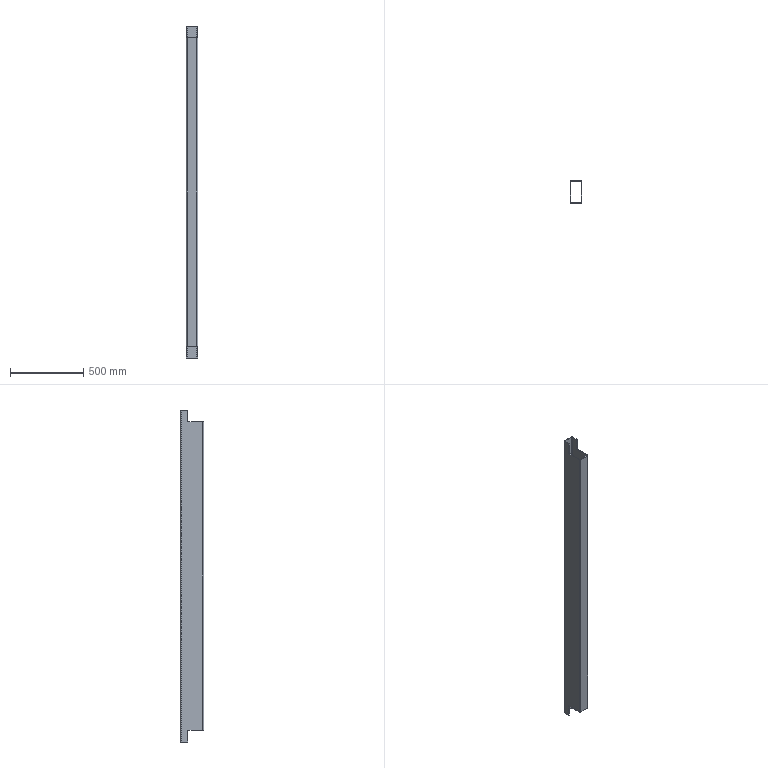Part | STEP file | 750078112 | 1 solid | 24 faces | box 80 x 160 x 2272 mm | volume 4914158 mm3 | plane 16 | cylinder 8 | commonest cylinder face diameters 4 x4 14 x4
STEP:
#1=CARTESIAN_POINT('',(-35.,-73.,1057.));
#2=VERTEX_POINT('',#1);
#3=CARTESIAN_POINT('',(-35.,28.5,1057.));
#4=VERTEX_POINT('',#3);
#5=CARTESIAN_POINT('',(-35.,-73.,1057.));
#6=DIRECTION('',(0.,1.,0.));
#7=VECTOR('',#6,1000.);
#8=LINE('',#5,#7);
#9=EDGE_CURVE('',#2,#4,#8,.T.);
#10=ORIENTED_EDGE('',*,*,#9,.F.);
#11=CARTESIAN_POINT('',(-35.,-73.,-1057.));
#12=VERTEX_POINT('',#11);
#13=CARTESIAN_POINT('',(-35.,-73.,1136.));
#14=DIRECTION('',(0.,0.,1.));
#15=VECTOR('',#14,1000.);
#16=LINE('',#13,#15);
#17=EDGE_CURVE('',#12,#2,#16,.T.);
#18=ORIENTED_EDGE('',*,*,#17,.F.);
#19=CARTESIAN_POINT('',(-35.,28.5,-1057.));
#20=VERTEX_POINT('',#19);
#21=CARTESIAN_POINT('',(-35.,-73.,-1057.));
#22=DIRECTION('',(0.,-1.,0.));
#23=VECTOR('',#22,1000.);
#24=LINE('',#21,#23);
#25=EDGE_CURVE('',#20,#12,#24,.T.);
#26=ORIENTED_EDGE('',*,*,#25,.F.);
#27=CARTESIAN_POINT('',(-35.,28.5,-1136.));
#28=VERTEX_POINT('',#27);
#29=CARTESIAN_POINT('',(-35.,28.5,1136.));
#30=DIRECTION('',(0.,0.,1.));
#31=VECTOR('',#30,1000.);
#32=LINE('',#29,#31);
#33=EDGE_CURVE('',#28,#20,#32,.T.);
#34=ORIENTED_EDGE('',*,*,#33,.F.);
#35=CARTESIAN_POINT('',(-35.,73.,-1136.));
#36=VERTEX_POINT('',#35);
#37=CARTESIAN_POINT('',(-35.,-73.,-1136.));
#38=DIRECTION('',(0.,-1.,0.));
#39=VECTOR('',#38,1000.);
#40=LINE('',#37,#39);
#41=EDGE_CURVE('',#36,#28,#40,.T.);
#42=ORIENTED_EDGE('',*,*,#41,.F.);
#43=CARTESIAN_POINT('',(-35.,73.,1136.));
#44=VERTEX_POINT('',#43);
#45=CARTESIAN_POINT('',(-35.,73.,1136.));
#46=DIRECTION('',(0.,0.,-1.));
#47=VECTOR('',#46,1000.);
#48=LINE('',#45,#47);
#49=EDGE_CURVE('',#44,#36,#48,.T.);
#50=ORIENTED_EDGE('',*,*,#49,.F.);
#51=CARTESIAN_POINT('',(-35.,28.5,1136.));
#52=VERTEX_POINT('',#51);
#53=CARTESIAN_POINT('',(-35.,-73.,1136.));
#54=DIRECTION('',(0.,1.,0.));
#55=VECTOR('',#54,1000.);
#56=LINE('',#53,#55);
#57=EDGE_CURVE('',#52,#44,#56,.T.);
#58=ORIENTED_EDGE('',*,*,#57,.F.);
#59=CARTESIAN_POINT('',(-35.,28.5,1136.));
#60=DIRECTION('',(0.,0.,1.));
#61=VECTOR('',#60,1000.);
#62=LINE('',#59,#61);
#63=EDGE_CURVE('',#4,#52,#62,.T.);
#64=ORIENTED_EDGE('',*,*,#63,.F.);
#65=EDGE_LOOP('',(#10,#18,#26,#34,#42,#50,#58,#64));
#66=FACE_OUTER_BOUND('',#65,.T.);
#67=CARTESIAN_POINT('',(-35.,-73.,1136.));
#68=DIRECTION('',(-1.,0.,0.));
#69=DIRECTION('',(0.,-1.,0.));
#70=AXIS2_PLACEMENT_3D('',#67,#68,#69);
#71=PLANE('',#70);
#72=ADVANCED_FACE('',(#66),#71,.F.);
#73=CARTESIAN_POINT('',(-40.,28.5,1057.));
#74=VERTEX_POINT('',#73);
#75=CARTESIAN_POINT('',(-40.,28.5,1136.));
#76=VERTEX_POINT('',#75);
#77=CARTESIAN_POINT('',(-40.,28.5,1057.));
#78=DIRECTION('',(0.,0.,1.));
#79=VECTOR('',#78,1000.);
#80=LINE('',#77,#79);
#81=EDGE_CURVE('',#74,#76,#80,.T.);
#82=ORIENTED_EDGE('',*,*,#81,.F.);
#83=CARTESIAN_POINT('',(-54960.,28.5,1057.));
#84=DIRECTION('',(-1.,0.,0.));
#85=VECTOR('',#84,1000.);
#86=LINE('',#83,#85);
#87=EDGE_CURVE('',#4,#74,#86,.T.);
#88=ORIENTED_EDGE('',*,*,#87,.F.);
#89=ORIENTED_EDGE('',*,*,#63,.T.);
#90=CARTESIAN_POINT('',(-54960.,28.5,1136.));
#91=DIRECTION('',(1.,0.,0.));
#92=VECTOR('',#91,1000.);
#93=LINE('',#90,#92);
#94=EDGE_CURVE('',#76,#52,#93,.T.);
#95=ORIENTED_EDGE('',*,*,#94,.F.);
#96=EDGE_LOOP('',(#82,#88,#89,#95));
#97=FACE_OUTER_BOUND('',#96,.T.);
#98=CARTESIAN_POINT('',(-54960.,28.5,1057.));
#99=DIRECTION('',(0.,1.,0.));
#100=DIRECTION('',(-1.,0.,0.));
#101=AXIS2_PLACEMENT_3D('',#98,#99,#100);
#102=PLANE('',#101);
#103=ADVANCED_FACE('',(#97),#102,.F.);
#104=CARTESIAN_POINT('',(-40.,-73.,1057.));
#105=VERTEX_POINT('',#104);
#106=CARTESIAN_POINT('',(-40.,-80.,1057.));
#107=DIRECTION('',(0.,1.,0.));
#108=VECTOR('',#107,1000.);
#109=LINE('',#106,#108);
#110=EDGE_CURVE('',#105,#74,#109,.T.);
#111=ORIENTED_EDGE('',*,*,#110,.F.);
#112=CARTESIAN_POINT('',(-33.,-80.,1057.));
#113=VERTEX_POINT('',#112);
#114=CARTESIAN_POINT('',(-33.,-73.,1057.));
#115=DIRECTION('',(0.,0.,-1.));
#116=DIRECTION('',(-1.,0.,0.));
#117=AXIS2_PLACEMENT_3D('',#114,#115,#116);
#118=CIRCLE('',#117,7.);
#119=EDGE_CURVE('',#113,#105,#118,.T.);
#120=ORIENTED_EDGE('',*,*,#119,.F.);
#121=CARTESIAN_POINT('',(33.,-80.,1057.));
#122=VERTEX_POINT('',#121);
#123=CARTESIAN_POINT('',(-54960.,-80.,1057.));
#124=DIRECTION('',(-1.,0.,0.));
#125=VECTOR('',#124,1000.);
#126=LINE('',#123,#125);
#127=EDGE_CURVE('',#122,#113,#126,.T.);
#128=ORIENTED_EDGE('',*,*,#127,.F.);
#129=CARTESIAN_POINT('',(40.,-73.,1057.));
#130=VERTEX_POINT('',#129);
#131=CARTESIAN_POINT('',(33.,-73.,1057.));
#132=DIRECTION('',(0.,0.,-1.));
#133=DIRECTION('',(-1.,0.,0.));
#134=AXIS2_PLACEMENT_3D('',#131,#132,#133);
#135=CIRCLE('',#134,7.);
#136=EDGE_CURVE('',#130,#122,#135,.T.);
#137=ORIENTED_EDGE('',*,*,#136,.F.);
#138=CARTESIAN_POINT('',(40.,28.5,1057.));
#139=VERTEX_POINT('',#138);
#140=CARTESIAN_POINT('',(40.,-80.,1057.));
#141=DIRECTION('',(0.,-1.,0.));
#142=VECTOR('',#141,1000.);
#143=LINE('',#140,#142);
#144=EDGE_CURVE('',#139,#130,#143,.T.);
#145=ORIENTED_EDGE('',*,*,#144,.F.);
#146=CARTESIAN_POINT('',(35.,28.5,1057.));
#147=VERTEX_POINT('',#146);
#148=CARTESIAN_POINT('',(-54960.,28.5,1057.));
#149=DIRECTION('',(1.,0.,0.));
#150=VECTOR('',#149,1000.);
#151=LINE('',#148,#150);
#152=EDGE_CURVE('',#147,#139,#151,.T.);
#153=ORIENTED_EDGE('',*,*,#152,.F.);
#154=CARTESIAN_POINT('',(35.,-73.,1057.));
#155=VERTEX_POINT('',#154);
#156=CARTESIAN_POINT('',(35.,-80.,1057.));
#157=DIRECTION('',(0.,1.,0.));
#158=VECTOR('',#157,1000.);
#159=LINE('',#156,#158);
#160=EDGE_CURVE('',#155,#147,#159,.T.);
#161=ORIENTED_EDGE('',*,*,#160,.F.);
#162=CARTESIAN_POINT('',(33.,-75.,1057.));
#163=VERTEX_POINT('',#162);
#164=CARTESIAN_POINT('',(33.,-73.,1057.));
#165=DIRECTION('',(0.,0.,1.));
#166=DIRECTION('',(-1.,0.,0.));
#167=AXIS2_PLACEMENT_3D('',#164,#165,#166);
#168=CIRCLE('',#167,2.);
#169=EDGE_CURVE('',#163,#155,#168,.T.);
#170=ORIENTED_EDGE('',*,*,#169,.F.);
#171=CARTESIAN_POINT('',(-33.,-75.,1057.));
#172=VERTEX_POINT('',#171);
#173=CARTESIAN_POINT('',(-54960.,-75.,1057.));
#174=DIRECTION('',(1.,0.,0.));
#175=VECTOR('',#174,1000.);
#176=LINE('',#173,#175);
#177=EDGE_CURVE('',#172,#163,#176,.T.);
#178=ORIENTED_EDGE('',*,*,#177,.F.);
#179=CARTESIAN_POINT('',(-33.,-73.,1057.));
#180=DIRECTION('',(0.,0.,1.));
#181=DIRECTION('',(-1.,0.,0.));
#182=AXIS2_PLACEMENT_3D('',#179,#180,#181);
#183=CIRCLE('',#182,2.);
#184=EDGE_CURVE('',#2,#172,#183,.T.);
#185=ORIENTED_EDGE('',*,*,#184,.F.);
#186=ORIENTED_EDGE('',*,*,#9,.T.);
#187=ORIENTED_EDGE('',*,*,#87,.T.);
#188=EDGE_LOOP('',(#111,#120,#128,#137,#145,#153,#161,#170,#178,#185,#186,#187));
#189=FACE_OUTER_BOUND('',#188,.T.);
#190=CARTESIAN_POINT('',(-54960.,-80.,1057.));
#191=DIRECTION('',(0.,0.,-1.));
#192=DIRECTION('',(0.,1.,0.));
#193=AXIS2_PLACEMENT_3D('',#190,#191,#192);
#194=PLANE('',#193);
#195=ADVANCED_FACE('',(#189),#194,.F.);
#196=ORIENTED_EDGE('',*,*,#184,.T.);
#197=CARTESIAN_POINT('',(-33.,-75.,-1057.));
#198=VERTEX_POINT('',#197);
#199=CARTESIAN_POINT('',(-33.,-75.,1136.));
#200=DIRECTION('',(0.,0.,1.));
#201=VECTOR('',#200,1000.);
#202=LINE('',#199,#201);
#203=EDGE_CURVE('',#198,#172,#202,.T.);
#204=ORIENTED_EDGE('',*,*,#203,.F.);
#205=CARTESIAN_POINT('',(-33.,-73.,-1057.));
#206=DIRECTION('',(0.,0.,1.));
#207=DIRECTION('',(-1.,0.,0.));
#208=AXIS2_PLACEMENT_3D('',#205,#206,#207);
#209=CIRCLE('',#208,2.);
#210=EDGE_CURVE('',#12,#198,#209,.T.);
#211=ORIENTED_EDGE('',*,*,#210,.F.);
#212=ORIENTED_EDGE('',*,*,#17,.T.);
#213=EDGE_LOOP('',(#196,#204,#211,#212));
#214=FACE_OUTER_BOUND('',#213,.T.);
#215=CARTESIAN_POINT('',(-33.,-73.,1136.));
#216=DIRECTION('',(0.,0.,-1.));
#217=DIRECTION('',(-1.,0.,0.));
#218=AXIS2_PLACEMENT_3D('',#215,#216,#217);
#219=CYLINDRICAL_SURFACE('',#218,2.);
#220=ADVANCED_FACE('',(#214),#219,.F.);
#221=CARTESIAN_POINT('',(33.,-75.,-1057.));
#222=VERTEX_POINT('',#221);
#223=CARTESIAN_POINT('',(-54960.,-75.,-1057.));
#224=DIRECTION('',(-1.,0.,0.));
#225=VECTOR('',#224,1000.);
#226=LINE('',#223,#225);
#227=EDGE_CURVE('',#222,#198,#226,.T.);
#228=ORIENTED_EDGE('',*,*,#227,.F.);
#229=CARTESIAN_POINT('',(35.,-73.,-1057.));
#230=VERTEX_POINT('',#229);
#231=CARTESIAN_POINT('',(33.,-73.,-1057.));
#232=DIRECTION('',(0.,0.,-1.));
#233=DIRECTION('',(-1.,0.,0.));
#234=AXIS2_PLACEMENT_3D('',#231,#232,#233);
#235=CIRCLE('',#234,2.);
#236=EDGE_CURVE('',#230,#222,#235,.T.);
#237=ORIENTED_EDGE('',*,*,#236,.F.);
#238=CARTESIAN_POINT('',(35.,28.5,-1057.));
#239=VERTEX_POINT('',#238);
#240=CARTESIAN_POINT('',(35.,28.5,-1057.));
#241=DIRECTION('',(0.,-1.,0.));
#242=VECTOR('',#241,1000.);
#243=LINE('',#240,#242);
#244=EDGE_CURVE('',#239,#230,#243,.T.);
#245=ORIENTED_EDGE('',*,*,#244,.F.);
#246=CARTESIAN_POINT('',(40.,28.5,-1057.));
#247=VERTEX_POINT('',#246);
#248=CARTESIAN_POINT('',(-54960.,28.5,-1057.));
#249=DIRECTION('',(-1.,0.,0.));
#250=VECTOR('',#249,1000.);
#251=LINE('',#248,#250);
#252=EDGE_CURVE('',#247,#239,#251,.T.);
#253=ORIENTED_EDGE('',*,*,#252,.F.);
#254=CARTESIAN_POINT('',(40.,-73.,-1057.));
#255=VERTEX_POINT('',#254);
#256=CARTESIAN_POINT('',(40.,28.5,-1057.));
#257=DIRECTION('',(0.,1.,0.));
#258=VECTOR('',#257,1000.);
#259=LINE('',#256,#258);
#260=EDGE_CURVE('',#255,#247,#259,.T.);
#261=ORIENTED_EDGE('',*,*,#260,.F.);
#262=CARTESIAN_POINT('',(33.,-80.,-1057.));
#263=VERTEX_POINT('',#262);
#264=CARTESIAN_POINT('',(33.,-73.,-1057.));
#265=DIRECTION('',(0.,0.,1.));
#266=DIRECTION('',(-1.,0.,0.));
#267=AXIS2_PLACEMENT_3D('',#264,#265,#266);
#268=CIRCLE('',#267,7.);
#269=EDGE_CURVE('',#263,#255,#268,.T.);
#270=ORIENTED_EDGE('',*,*,#269,.F.);
#271=CARTESIAN_POINT('',(-33.,-80.,-1057.));
#272=VERTEX_POINT('',#271);
#273=CARTESIAN_POINT('',(-54960.,-80.,-1057.));
#274=DIRECTION('',(1.,0.,0.));
#275=VECTOR('',#274,1000.);
#276=LINE('',#273,#275);
#277=EDGE_CURVE('',#272,#263,#276,.T.);
#278=ORIENTED_EDGE('',*,*,#277,.F.);
#279=CARTESIAN_POINT('',(-40.,-73.,-1057.));
#280=VERTEX_POINT('',#279);
#281=CARTESIAN_POINT('',(-33.,-73.,-1057.));
#282=DIRECTION('',(0.,0.,1.));
#283=DIRECTION('',(-1.,0.,0.));
#284=AXIS2_PLACEMENT_3D('',#281,#282,#283);
#285=CIRCLE('',#284,7.);
#286=EDGE_CURVE('',#280,#272,#285,.T.);
#287=ORIENTED_EDGE('',*,*,#286,.F.);
#288=CARTESIAN_POINT('',(-40.,28.5,-1057.));
#289=VERTEX_POINT('',#288);
#290=CARTESIAN_POINT('',(-40.,28.5,-1057.));
#291=DIRECTION('',(0.,-1.,0.));
#292=VECTOR('',#291,1000.);
#293=LINE('',#290,#292);
#294=EDGE_CURVE('',#289,#280,#293,.T.);
#295=ORIENTED_EDGE('',*,*,#294,.F.);
#296=CARTESIAN_POINT('',(-54960.,28.5,-1057.));
#297=DIRECTION('',(-1.,0.,0.));
#298=VECTOR('',#297,1000.);
#299=LINE('',#296,#298);
#300=EDGE_CURVE('',#20,#289,#299,.T.);
#301=ORIENTED_EDGE('',*,*,#300,.F.);
#302=ORIENTED_EDGE('',*,*,#25,.T.);
#303=ORIENTED_EDGE('',*,*,#210,.T.);
#304=EDGE_LOOP('',(#228,#237,#245,#253,#261,#270,#278,#287,#295,#301,#302,#303));
#305=FACE_OUTER_BOUND('',#304,.T.);
#306=CARTESIAN_POINT('',(-54960.,28.5,-1057.));
#307=DIRECTION('',(0.,0.,1.));
#308=DIRECTION('',(0.,-1.,0.));
#309=AXIS2_PLACEMENT_3D('',#306,#307,#308);
#310=PLANE('',#309);
#311=ADVANCED_FACE('',(#305),#310,.F.);
#312=CARTESIAN_POINT('',(-40.,28.5,-1136.));
#313=VERTEX_POINT('',#312);
#314=CARTESIAN_POINT('',(-40.,28.5,-1136.));
#315=DIRECTION('',(0.,0.,1.));
#316=VECTOR('',#315,1000.);
#317=LINE('',#314,#316);
#318=EDGE_CURVE('',#313,#289,#317,.T.);
#319=ORIENTED_EDGE('',*,*,#318,.F.);
#320=CARTESIAN_POINT('',(-54960.,28.5,-1136.));
#321=DIRECTION('',(-1.,0.,0.));
#322=VECTOR('',#321,1000.);
#323=LINE('',#320,#322);
#324=EDGE_CURVE('',#28,#313,#323,.T.);
#325=ORIENTED_EDGE('',*,*,#324,.F.);
#326=ORIENTED_EDGE('',*,*,#33,.T.);
#327=ORIENTED_EDGE('',*,*,#300,.T.);
#328=EDGE_LOOP('',(#319,#325,#326,#327));
#329=FACE_OUTER_BOUND('',#328,.T.);
#330=CARTESIAN_POINT('',(-54960.,28.5,-1136.));
#331=DIRECTION('',(0.,1.,0.));
#332=DIRECTION('',(-1.,0.,0.));
#333=AXIS2_PLACEMENT_3D('',#330,#331,#332);
#334=PLANE('',#333);
#335=ADVANCED_FACE('',(#329),#334,.F.);
#336=CARTESIAN_POINT('',(-33.,75.,-1136.));
#337=VERTEX_POINT('',#336);
#338=CARTESIAN_POINT('',(-33.,73.,-1136.));
#339=DIRECTION('',(0.,0.,1.));
#340=DIRECTION('',(-1.,0.,0.));
#341=AXIS2_PLACEMENT_3D('',#338,#339,#340);
#342=CIRCLE('',#341,2.);
#343=EDGE_CURVE('',#337,#36,#342,.T.);
#344=ORIENTED_EDGE('',*,*,#343,.T.);
#345=ORIENTED_EDGE('',*,*,#41,.T.);
#346=ORIENTED_EDGE('',*,*,#324,.T.);
#347=CARTESIAN_POINT('',(-40.,73.,-1136.));
#348=VERTEX_POINT('',#347);
#349=CARTESIAN_POINT('',(-40.,-73.,-1136.));
#350=DIRECTION('',(0.,1.,0.));
#351=VECTOR('',#350,1000.);
#352=LINE('',#349,#351);
#353=EDGE_CURVE('',#313,#348,#352,.T.);
#354=ORIENTED_EDGE('',*,*,#353,.T.);
#355=CARTESIAN_POINT('',(-33.,80.,-1136.));
#356=VERTEX_POINT('',#355);
#357=CARTESIAN_POINT('',(-33.,73.,-1136.));
#358=DIRECTION('',(0.,0.,-1.));
#359=DIRECTION('',(-1.,0.,0.));
#360=AXIS2_PLACEMENT_3D('',#357,#358,#359);
#361=CIRCLE('',#360,7.);
#362=EDGE_CURVE('',#348,#356,#361,.T.);
#363=ORIENTED_EDGE('',*,*,#362,.T.);
#364=CARTESIAN_POINT('',(33.,80.,-1136.));
#365=VERTEX_POINT('',#364);
#366=CARTESIAN_POINT('',(33.,80.,-1136.));
#367=DIRECTION('',(1.,0.,0.));
#368=VECTOR('',#367,1000.);
#369=LINE('',#366,#368);
#370=EDGE_CURVE('',#356,#365,#369,.T.);
#371=ORIENTED_EDGE('',*,*,#370,.T.);
#372=CARTESIAN_POINT('',(40.,73.,-1136.));
#373=VERTEX_POINT('',#372);
#374=CARTESIAN_POINT('',(33.,73.,-1136.));
#375=DIRECTION('',(0.,0.,-1.));
#376=DIRECTION('',(-1.,0.,0.));
#377=AXIS2_PLACEMENT_3D('',#374,#375,#376);
#378=CIRCLE('',#377,7.);
#379=EDGE_CURVE('',#365,#373,#378,.T.);
#380=ORIENTED_EDGE('',*,*,#379,.T.);
#381=CARTESIAN_POINT('',(40.,28.5,-1136.));
#382=VERTEX_POINT('',#381);
#383=CARTESIAN_POINT('',(40.,-73.,-1136.));
#384=DIRECTION('',(0.,-1.,0.));
#385=VECTOR('',#384,1000.);
#386=LINE('',#383,#385);
#387=EDGE_CURVE('',#373,#382,#386,.T.);
#388=ORIENTED_EDGE('',*,*,#387,.T.);
#389=CARTESIAN_POINT('',(35.,28.5,-1136.));
#390=VERTEX_POINT('',#389);
#391=CARTESIAN_POINT('',(33.,28.5,-1136.));
#392=DIRECTION('',(-1.,0.,0.));
#393=VECTOR('',#392,1000.);
#394=LINE('',#391,#393);
#395=EDGE_CURVE('',#382,#390,#394,.T.);
#396=ORIENTED_EDGE('',*,*,#395,.T.);
#397=CARTESIAN_POINT('',(35.,73.,-1136.));
#398=VERTEX_POINT('',#397);
#399=CARTESIAN_POINT('',(35.,-73.,-1136.));
#400=DIRECTION('',(0.,1.,0.));
#401=VECTOR('',#400,1000.);
#402=LINE('',#399,#401);
#403=EDGE_CURVE('',#390,#398,#402,.T.);
#404=ORIENTED_EDGE('',*,*,#403,.T.);
#405=CARTESIAN_POINT('',(33.,75.,-1136.));
#406=VERTEX_POINT('',#405);
#407=CARTESIAN_POINT('',(33.,73.,-1136.));
#408=DIRECTION('',(0.,0.,1.));
#409=DIRECTION('',(-1.,0.,0.));
#410=AXIS2_PLACEMENT_3D('',#407,#408,#409);
#411=CIRCLE('',#410,2.);
#412=EDGE_CURVE('',#398,#406,#411,.T.);
#413=ORIENTED_EDGE('',*,*,#412,.T.);
#414=CARTESIAN_POINT('',(33.,75.,-1136.));
#415=DIRECTION('',(-1.,0.,0.));
#416=VECTOR('',#415,1000.);
#417=LINE('',#414,#416);
#418=EDGE_CURVE('',#406,#337,#417,.T.);
#419=ORIENTED_EDGE('',*,*,#418,.T.);
#420=EDGE_LOOP('',(#344,#345,#346,#354,#363,#371,#380,#388,#396,#404,#413,#419));
#421=FACE_OUTER_BOUND('',#420,.T.);
#422=CARTESIAN_POINT('',(33.,-73.,-1136.));
#423=DIRECTION('',(0.,0.,-1.));
#424=DIRECTION('',(-1.,0.,0.));
#425=AXIS2_PLACEMENT_3D('',#422,#423,#424);
#426=PLANE('',#425);
#427=ADVANCED_FACE('',(#421),#426,.T.);
#428=CARTESIAN_POINT('',(-33.,75.,1136.));
#429=VERTEX_POINT('',#428);
#430=CARTESIAN_POINT('',(-33.,75.,1136.));
#431=DIRECTION('',(0.,0.,-1.));
#432=VECTOR('',#431,1000.);
#433=LINE('',#430,#432);
#434=EDGE_CURVE('',#429,#337,#433,.T.);
#435=ORIENTED_EDGE('',*,*,#434,.F.);
#436=CARTESIAN_POINT('',(-33.,73.,1136.));
#437=DIRECTION('',(0.,0.,-1.));
#438=DIRECTION('',(-1.,0.,0.));
#439=AXIS2_PLACEMENT_3D('',#436,#437,#438);
#440=CIRCLE('',#439,2.);
#441=EDGE_CURVE('',#44,#429,#440,.T.);
#442=ORIENTED_EDGE('',*,*,#441,.F.);
#443=ORIENTED_EDGE('',*,*,#49,.T.);
#444=ORIENTED_EDGE('',*,*,#343,.F.);
#445=EDGE_LOOP('',(#435,#442,#443,#444));
#446=FACE_OUTER_BOUND('',#445,.T.);
#447=CARTESIAN_POINT('',(-33.,73.,1136.));
#448=DIRECTION('',(0.,0.,-1.));
#449=DIRECTION('',(-1.,0.,0.));
#450=AXIS2_PLACEMENT_3D('',#447,#448,#449);
#451=CYLINDRICAL_SURFACE('',#450,2.);
#452=ADVANCED_FACE('',(#446),#451,.F.);
#453=ORIENTED_EDGE('',*,*,#94,.T.);
#454=ORIENTED_EDGE('',*,*,#57,.T.);
#455=ORIENTED_EDGE('',*,*,#441,.T.);
#456=CARTESIAN_POINT('',(33.,75.,1136.));
#457=VERTEX_POINT('',#456);
#458=CARTESIAN_POINT('',(33.,75.,1136.));
#459=DIRECTION('',(-1.,0.,0.));
#460=VECTOR('',#459,1000.);
#461=LINE('',#458,#460);
#462=EDGE_CURVE('',#457,#429,#461,.T.);
#463=ORIENTED_EDGE('',*,*,#462,.F.);
#464=CARTESIAN_POINT('',(35.,73.,1136.));
#465=VERTEX_POINT('',#464);
#466=CARTESIAN_POINT('',(33.,73.,1136.));
#467=DIRECTION('',(0.,0.,1.));
#468=DIRECTION('',(-1.,0.,0.));
#469=AXIS2_PLACEMENT_3D('',#466,#467,#468);
#470=CIRCLE('',#469,2.);
#471=EDGE_CURVE('',#465,#457,#470,.T.);
#472=ORIENTED_EDGE('',*,*,#471,.F.);
#473=CARTESIAN_POINT('',(35.,28.5,1136.));
#474=VERTEX_POINT('',#473);
#475=CARTESIAN_POINT('',(35.,-73.,1136.));
#476=DIRECTION('',(0.,1.,0.));
#477=VECTOR('',#476,1000.);
#478=LINE('',#475,#477);
#479=EDGE_CURVE('',#474,#465,#478,.T.);
#480=ORIENTED_EDGE('',*,*,#479,.F.);
#481=CARTESIAN_POINT('',(40.,28.5,1136.));
#482=VERTEX_POINT('',#481);
#483=CARTESIAN_POINT('',(33.,28.5,1136.));
#484=DIRECTION('',(-1.,0.,0.));
#485=VECTOR('',#484,1000.);
#486=LINE('',#483,#485);
#487=EDGE_CURVE('',#482,#474,#486,.T.);
#488=ORIENTED_EDGE('',*,*,#487,.F.);
#489=CARTESIAN_POINT('',(40.,73.,1136.));
#490=VERTEX_POINT('',#489);
#491=CARTESIAN_POINT('',(40.,-73.,1136.));
#492=DIRECTION('',(0.,-1.,0.));
#493=VECTOR('',#492,1000.);
#494=LINE('',#491,#493);
#495=EDGE_CURVE('',#490,#482,#494,.T.);
#496=ORIENTED_EDGE('',*,*,#495,.F.);
#497=CARTESIAN_POINT('',(33.,80.,1136.));
#498=VERTEX_POINT('',#497);
#499=CARTESIAN_POINT('',(33.,73.,1136.));
#500=DIRECTION('',(0.,0.,-1.));
#501=DIRECTION('',(-1.,0.,0.));
#502=AXIS2_PLACEMENT_3D('',#499,#500,#501);
#503=CIRCLE('',#502,7.);
#504=EDGE_CURVE('',#498,#490,#503,.T.);
#505=ORIENTED_EDGE('',*,*,#504,.F.);
#506=CARTESIAN_POINT('',(-33.,80.,1136.));
#507=VERTEX_POINT('',#506);
#508=CARTESIAN_POINT('',(33.,80.,1136.));
#509=DIRECTION('',(1.,0.,0.));
#510=VECTOR('',#509,1000.);
#511=LINE('',#508,#510);
#512=EDGE_CURVE('',#507,#498,#511,.T.);
#513=ORIENTED_EDGE('',*,*,#512,.F.);
#514=CARTESIAN_POINT('',(-40.,73.,1136.));
#515=VERTEX_POINT('',#514);
#516=CARTESIAN_POINT('',(-33.,73.,1136.));
#517=DIRECTION('',(0.,0.,-1.));
#518=DIRECTION('',(-1.,0.,0.));
#519=AXIS2_PLACEMENT_3D('',#516,#517,#518);
#520=CIRCLE('',#519,7.);
#521=EDGE_CURVE('',#515,#507,#520,.T.);
#522=ORIENTED_EDGE('',*,*,#521,.F.);
#523=CARTESIAN_POINT('',(-40.,-73.,1136.));
#524=DIRECTION('',(0.,1.,0.));
#525=VECTOR('',#524,1000.);
#526=LINE('',#523,#525);
#527=EDGE_CURVE('',#76,#515,#526,.T.);
#528=ORIENTED_EDGE('',*,*,#527,.F.);
#529=EDGE_LOOP('',(#453,#454,#455,#463,#472,#480,#488,#496,#505,#513,#522,#528));
#530=FACE_OUTER_BOUND('',#529,.T.);
#531=CARTESIAN_POINT('',(33.,-73.,1136.));
#532=DIRECTION('',(0.,0.,-1.));
#533=DIRECTION('',(-1.,0.,0.));
#534=AXIS2_PLACEMENT_3D('',#531,#532,#533);
#535=PLANE('',#534);
#536=ADVANCED_FACE('',(#530),#535,.F.);
#537=ORIENTED_EDGE('',*,*,#294,.T.);
#538=CARTESIAN_POINT('',(-40.,-73.,1136.));
#539=DIRECTION('',(0.,0.,1.));
#540=VECTOR('',#539,1000.);
#541=LINE('',#538,#540);
#542=EDGE_CURVE('',#280,#105,#541,.T.);
#543=ORIENTED_EDGE('',*,*,#542,.T.);
#544=ORIENTED_EDGE('',*,*,#110,.T.);
#545=ORIENTED_EDGE('',*,*,#81,.T.);
#546=ORIENTED_EDGE('',*,*,#527,.T.);
#547=CARTESIAN_POINT('',(-40.,73.,1136.));
#548=DIRECTION('',(0.,0.,-1.));
#549=VECTOR('',#548,1000.);
#550=LINE('',#547,#549);
#551=EDGE_CURVE('',#515,#348,#550,.T.);
#552=ORIENTED_EDGE('',*,*,#551,.T.);
#553=ORIENTED_EDGE('',*,*,#353,.F.);
#554=ORIENTED_EDGE('',*,*,#318,.T.);
#555=EDGE_LOOP('',(#537,#543,#544,#545,#546,#552,#553,#554));
#556=FACE_OUTER_BOUND('',#555,.T.);
#557=CARTESIAN_POINT('',(-40.,-73.,1136.));
#558=DIRECTION('',(-1.,0.,0.));
#559=DIRECTION('',(0.,0.,1.));
#560=AXIS2_PLACEMENT_3D('',#557,#558,#559);
#561=PLANE('',#560);
#562=ADVANCED_FACE('',(#556),#561,.T.);
#563=ORIENTED_EDGE('',*,*,#286,.T.);
#564=CARTESIAN_POINT('',(-33.,-80.,1136.));
#565=DIRECTION('',(0.,0.,1.));
#566=VECTOR('',#565,1000.);
#567=LINE('',#564,#566);
#568=EDGE_CURVE('',#272,#113,#567,.T.);
#569=ORIENTED_EDGE('',*,*,#568,.T.);
#570=ORIENTED_EDGE('',*,*,#119,.T.);
#571=ORIENTED_EDGE('',*,*,#542,.F.);
#572=EDGE_LOOP('',(#563,#569,#570,#571));
#573=FACE_OUTER_BOUND('',#572,.T.);
#574=CARTESIAN_POINT('',(-33.,-73.,1136.));
#575=DIRECTION('',(0.,0.,-1.));
#576=DIRECTION('',(-1.,0.,0.));
#577=AXIS2_PLACEMENT_3D('',#574,#575,#576);
#578=CYLINDRICAL_SURFACE('',#577,7.);
#579=ADVANCED_FACE('',(#573),#578,.T.);
#580=ORIENTED_EDGE('',*,*,#277,.T.);
#581=CARTESIAN_POINT('',(33.,-80.,1136.));
#582=DIRECTION('',(0.,0.,1.));
#583=VECTOR('',#582,1000.);
#584=LINE('',#581,#583);
#585=EDGE_CURVE('',#263,#122,#584,.T.);
#586=ORIENTED_EDGE('',*,*,#585,.T.);
#587=ORIENTED_EDGE('',*,*,#127,.T.);
#588=ORIENTED_EDGE('',*,*,#568,.F.);
#589=EDGE_LOOP('',(#580,#586,#587,#588));
#590=FACE_OUTER_BOUND('',#589,.T.);
#591=CARTESIAN_POINT('',(33.,-80.,1136.));
#592=DIRECTION('',(0.,-1.,0.));
#593=DIRECTION('',(0.,0.,-1.));
#594=AXIS2_PLACEMENT_3D('',#591,#592,#593);
#595=PLANE('',#594);
#596=ADVANCED_FACE('',(#590),#595,.T.);
#597=ORIENTED_EDGE('',*,*,#269,.T.);
#598=CARTESIAN_POINT('',(40.,-73.,1136.));
#599=DIRECTION('',(0.,0.,1.));
#600=VECTOR('',#599,1000.);
#601=LINE('',#598,#600);
#602=EDGE_CURVE('',#255,#130,#601,.T.);
#603=ORIENTED_EDGE('',*,*,#602,.T.);
#604=ORIENTED_EDGE('',*,*,#136,.T.);
#605=ORIENTED_EDGE('',*,*,#585,.F.);
#606=EDGE_LOOP('',(#597,#603,#604,#605));
#607=FACE_OUTER_BOUND('',#606,.T.);
#608=CARTESIAN_POINT('',(33.,-73.,1136.));
#609=DIRECTION('',(0.,0.,-1.));
#610=DIRECTION('',(-1.,0.,0.));
#611=AXIS2_PLACEMENT_3D('',#608,#609,#610);
#612=CYLINDRICAL_SURFACE('',#611,7.);
#613=ADVANCED_FACE('',(#607),#612,.T.);
#614=ORIENTED_EDGE('',*,*,#495,.T.);
#615=CARTESIAN_POINT('',(40.,28.5,1136.));
#616=DIRECTION('',(0.,0.,-1.));
#617=VECTOR('',#616,1000.);
#618=LINE('',#615,#617);
#619=EDGE_CURVE('',#482,#139,#618,.T.);
#620=ORIENTED_EDGE('',*,*,#619,.T.);
#621=ORIENTED_EDGE('',*,*,#144,.T.);
#622=ORIENTED_EDGE('',*,*,#602,.F.);
#623=ORIENTED_EDGE('',*,*,#260,.T.);
#624=CARTESIAN_POINT('',(40.,28.5,1136.));
#625=DIRECTION('',(0.,0.,-1.));
#626=VECTOR('',#625,1000.);
#627=LINE('',#624,#626);
#628=EDGE_CURVE('',#247,#382,#627,.T.);
#629=ORIENTED_EDGE('',*,*,#628,.T.);
#630=ORIENTED_EDGE('',*,*,#387,.F.);
#631=CARTESIAN_POINT('',(40.,73.,1136.));
#632=DIRECTION('',(0.,0.,1.));
#633=VECTOR('',#632,1000.);
#634=LINE('',#631,#633);
#635=EDGE_CURVE('',#373,#490,#634,.T.);
#636=ORIENTED_EDGE('',*,*,#635,.T.);
#637=EDGE_LOOP('',(#614,#620,#621,#622,#623,#629,#630,#636));
#638=FACE_OUTER_BOUND('',#637,.T.);
#639=CARTESIAN_POINT('',(40.,73.,1136.));
#640=DIRECTION('',(1.,0.,0.));
#641=DIRECTION('',(0.,1.,0.));
#642=AXIS2_PLACEMENT_3D('',#639,#640,#641);
#643=PLANE('',#642);
#644=ADVANCED_FACE('',(#638),#643,.T.);
#645=ORIENTED_EDGE('',*,*,#619,.F.);
#646=ORIENTED_EDGE('',*,*,#487,.T.);
#647=CARTESIAN_POINT('',(35.,28.5,1057.));
#648=DIRECTION('',(0.,0.,1.));
#649=VECTOR('',#648,1000.);
#650=LINE('',#647,#649);
#651=EDGE_CURVE('',#147,#474,#650,.T.);
#652=ORIENTED_EDGE('',*,*,#651,.F.);
#653=ORIENTED_EDGE('',*,*,#152,.T.);
#654=EDGE_LOOP('',(#645,#646,#652,#653));
#655=FACE_OUTER_BOUND('',#654,.T.);
#656=CARTESIAN_POINT('',(-54960.,28.5,1057.));
#657=DIRECTION('',(0.,1.,0.));
#658=DIRECTION('',(-1.,0.,0.));
#659=AXIS2_PLACEMENT_3D('',#656,#657,#658);
#660=PLANE('',#659);
#661=ADVANCED_FACE('',(#655),#660,.F.);
#662=ORIENTED_EDGE('',*,*,#160,.T.);
#663=ORIENTED_EDGE('',*,*,#651,.T.);
#664=ORIENTED_EDGE('',*,*,#479,.T.);
#665=CARTESIAN_POINT('',(35.,73.,1136.));
#666=DIRECTION('',(0.,0.,1.));
#667=VECTOR('',#666,1000.);
#668=LINE('',#665,#667);
#669=EDGE_CURVE('',#398,#465,#668,.T.);
#670=ORIENTED_EDGE('',*,*,#669,.F.);
#671=ORIENTED_EDGE('',*,*,#403,.F.);
#672=CARTESIAN_POINT('',(35.,28.5,1136.));
#673=DIRECTION('',(0.,0.,-1.));
#674=VECTOR('',#673,1000.);
#675=LINE('',#672,#674);
#676=EDGE_CURVE('',#239,#390,#675,.T.);
#677=ORIENTED_EDGE('',*,*,#676,.F.);
#678=ORIENTED_EDGE('',*,*,#244,.T.);
#679=CARTESIAN_POINT('',(35.,-73.,1136.));
#680=DIRECTION('',(0.,0.,-1.));
#681=VECTOR('',#680,1000.);
#682=LINE('',#679,#681);
#683=EDGE_CURVE('',#155,#230,#682,.T.);
#684=ORIENTED_EDGE('',*,*,#683,.F.);
#685=EDGE_LOOP('',(#662,#663,#664,#670,#671,#677,#678,#684));
#686=FACE_OUTER_BOUND('',#685,.T.);
#687=CARTESIAN_POINT('',(35.,73.,1136.));
#688=DIRECTION('',(1.,0.,0.));
#689=DIRECTION('',(0.,1.,0.));
#690=AXIS2_PLACEMENT_3D('',#687,#688,#689);
#691=PLANE('',#690);
#692=ADVANCED_FACE('',(#686),#691,.F.);
#693=ORIENTED_EDGE('',*,*,#169,.T.);
#694=ORIENTED_EDGE('',*,*,#683,.T.);
#695=ORIENTED_EDGE('',*,*,#236,.T.);
#696=CARTESIAN_POINT('',(33.,-75.,1136.));
#697=DIRECTION('',(0.,0.,-1.));
#698=VECTOR('',#697,1000.);
#699=LINE('',#696,#698);
#700=EDGE_CURVE('',#163,#222,#699,.T.);
#701=ORIENTED_EDGE('',*,*,#700,.F.);
#702=EDGE_LOOP('',(#693,#694,#695,#701));
#703=FACE_OUTER_BOUND('',#702,.T.);
#704=CARTESIAN_POINT('',(33.,-73.,1136.));
#705=DIRECTION('',(0.,0.,-1.));
#706=DIRECTION('',(-1.,0.,0.));
#707=AXIS2_PLACEMENT_3D('',#704,#705,#706);
#708=CYLINDRICAL_SURFACE('',#707,2.);
#709=ADVANCED_FACE('',(#703),#708,.F.);
#710=ORIENTED_EDGE('',*,*,#177,.T.);
#711=ORIENTED_EDGE('',*,*,#700,.T.);
#712=ORIENTED_EDGE('',*,*,#227,.T.);
#713=ORIENTED_EDGE('',*,*,#203,.T.);
#714=EDGE_LOOP('',(#710,#711,#712,#713));
#715=FACE_OUTER_BOUND('',#714,.T.);
#716=CARTESIAN_POINT('',(33.,-75.,1136.));
#717=DIRECTION('',(0.,-1.,0.));
#718=DIRECTION('',(0.,0.,-1.));
#719=AXIS2_PLACEMENT_3D('',#716,#717,#718);
#720=PLANE('',#719);
#721=ADVANCED_FACE('',(#715),#720,.F.);
#722=ORIENTED_EDGE('',*,*,#628,.F.);
#723=ORIENTED_EDGE('',*,*,#252,.T.);
#724=ORIENTED_EDGE('',*,*,#676,.T.);
#725=ORIENTED_EDGE('',*,*,#395,.F.);
#726=EDGE_LOOP('',(#722,#723,#724,#725));
#727=FACE_OUTER_BOUND('',#726,.T.);
#728=CARTESIAN_POINT('',(-54960.,28.5,-1136.));
#729=DIRECTION('',(0.,1.,0.));
#730=DIRECTION('',(-1.,0.,0.));
#731=AXIS2_PLACEMENT_3D('',#728,#729,#730);
#732=PLANE('',#731);
#733=ADVANCED_FACE('',(#727),#732,.F.);
#734=CARTESIAN_POINT('',(33.,75.,1136.));
#735=DIRECTION('',(0.,0.,-1.));
#736=VECTOR('',#735,1000.);
#737=LINE('',#734,#736);
#738=EDGE_CURVE('',#457,#406,#737,.T.);
#739=ORIENTED_EDGE('',*,*,#738,.F.);
#740=ORIENTED_EDGE('',*,*,#462,.T.);
#741=ORIENTED_EDGE('',*,*,#434,.T.);
#742=ORIENTED_EDGE('',*,*,#418,.F.);
#743=EDGE_LOOP('',(#739,#740,#741,#742));
#744=FACE_OUTER_BOUND('',#743,.T.);
#745=CARTESIAN_POINT('',(-33.,75.,1136.));
#746=DIRECTION('',(0.,1.,0.));
#747=DIRECTION('',(0.,0.,1.));
#748=AXIS2_PLACEMENT_3D('',#745,#746,#747);
#749=PLANE('',#748);
#750=ADVANCED_FACE('',(#744),#749,.F.);
#751=ORIENTED_EDGE('',*,*,#669,.T.);
#752=ORIENTED_EDGE('',*,*,#471,.T.);
#753=ORIENTED_EDGE('',*,*,#738,.T.);
#754=ORIENTED_EDGE('',*,*,#412,.F.);
#755=EDGE_LOOP('',(#751,#752,#753,#754));
#756=FACE_OUTER_BOUND('',#755,.T.);
#757=CARTESIAN_POINT('',(33.,73.,1136.));
#758=DIRECTION('',(0.,0.,-1.));
#759=DIRECTION('',(-1.,0.,0.));
#760=AXIS2_PLACEMENT_3D('',#757,#758,#759);
#761=CYLINDRICAL_SURFACE('',#760,2.);
#762=ADVANCED_FACE('',(#756),#761,.F.);
#763=ORIENTED_EDGE('',*,*,#504,.T.);
#764=ORIENTED_EDGE('',*,*,#635,.F.);
#765=ORIENTED_EDGE('',*,*,#379,.F.);
#766=CARTESIAN_POINT('',(33.,80.,1136.));
#767=DIRECTION('',(0.,0.,1.));
#768=VECTOR('',#767,1000.);
#769=LINE('',#766,#768);
#770=EDGE_CURVE('',#365,#498,#769,.T.);
#771=ORIENTED_EDGE('',*,*,#770,.T.);
#772=EDGE_LOOP('',(#763,#764,#765,#771));
#773=FACE_OUTER_BOUND('',#772,.T.);
#774=CARTESIAN_POINT('',(33.,73.,1136.));
#775=DIRECTION('',(0.,0.,-1.));
#776=DIRECTION('',(-1.,0.,0.));
#777=AXIS2_PLACEMENT_3D('',#774,#775,#776);
#778=CYLINDRICAL_SURFACE('',#777,7.);
#779=ADVANCED_FACE('',(#773),#778,.T.);
#780=ORIENTED_EDGE('',*,*,#512,.T.);
#781=ORIENTED_EDGE('',*,*,#770,.F.);
#782=ORIENTED_EDGE('',*,*,#370,.F.);
#783=CARTESIAN_POINT('',(-33.,80.,1136.));
#784=DIRECTION('',(0.,0.,1.));
#785=VECTOR('',#784,1000.);
#786=LINE('',#783,#785);
#787=EDGE_CURVE('',#356,#507,#786,.T.);
#788=ORIENTED_EDGE('',*,*,#787,.T.);
#789=EDGE_LOOP('',(#780,#781,#782,#788));
#790=FACE_OUTER_BOUND('',#789,.T.);
#791=CARTESIAN_POINT('',(-33.,80.,1136.));
#792=DIRECTION('',(0.,1.,0.));
#793=DIRECTION('',(0.,0.,1.));
#794=AXIS2_PLACEMENT_3D('',#791,#792,#793);
#795=PLANE('',#794);
#796=ADVANCED_FACE('',(#790),#795,.T.);
#797=ORIENTED_EDGE('',*,*,#521,.T.);
#798=ORIENTED_EDGE('',*,*,#787,.F.);
#799=ORIENTED_EDGE('',*,*,#362,.F.);
#800=ORIENTED_EDGE('',*,*,#551,.F.);
#801=EDGE_LOOP('',(#797,#798,#799,#800));
#802=FACE_OUTER_BOUND('',#801,.T.);
#803=CARTESIAN_POINT('',(-33.,73.,1136.));
#804=DIRECTION('',(0.,0.,-1.));
#805=DIRECTION('',(-1.,0.,0.));
#806=AXIS2_PLACEMENT_3D('',#803,#804,#805);
#807=CYLINDRICAL_SURFACE('',#806,7.);
#808=ADVANCED_FACE('',(#802),#807,.T.);
#809=CLOSED_SHELL('',(#72,#103,#195,#220,#311,#335,#427,#452,#536,#562,#579,#596,#613,#644,#661,#692,#709,#721,#733,#750,#762,#779,#796,#808));
#810=MANIFOLD_SOLID_BREP('',#809);
#811=CARTESIAN_POINT('',(0.,0.,0.));
#812=DIRECTION('',(0.,0.,1.));
#813=DIRECTION('',(1.,0.,0.));
#814=AXIS2_PLACEMENT_3D('',#811,#812,#813);
#815=(LENGTH_UNIT()NAMED_UNIT(*)SI_UNIT(.MILLI.,.METRE.));
#816=UNCERTAINTY_MEASURE_WITH_UNIT(LENGTH_MEASURE(0.00001),#815,'','');
#817=(NAMED_UNIT(*)PLANE_ANGLE_UNIT()SI_UNIT($,.RADIAN.));
#818=(NAMED_UNIT(*)SI_UNIT($,.STERADIAN.)SOLID_ANGLE_UNIT());
#819=(GEOMETRIC_REPRESENTATION_CONTEXT(3)GLOBAL_UNCERTAINTY_ASSIGNED_CONTEXT((#816))GLOBAL_UNIT_ASSIGNED_CONTEXT((#815,#817,#818))REPRESENTATION_CONTEXT('',''));
#820=ADVANCED_BREP_SHAPE_REPRESENTATION('',(#810,#814),#819);